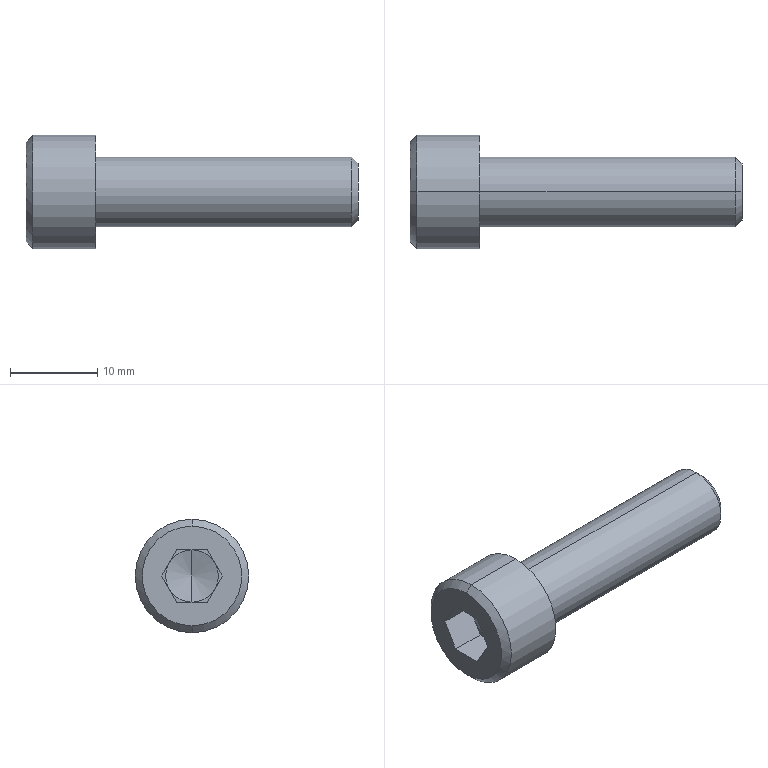Part | STEP file | 0244_305_SCB8-30 | 1 solid | 25 faces | box 38 x 13 x 13 mm | volume 2418 mm3 | plane 15 | cone 6 | cylinder 4 | commonest cylinder face diameters 8 x2 13 x2